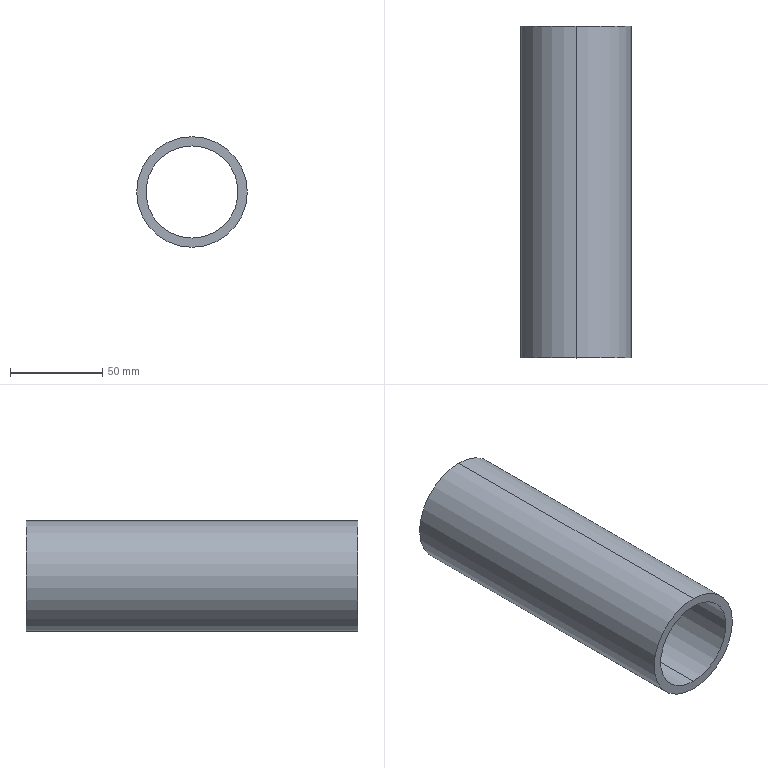Part | SolidWorks | features Extrusion 1 | 1 solid | 6 faces | box 60 x 180 x 60 mm | volume 155509 mm3 | cylinder 4 | plane 2 | commonest cylinder face diameters 50 x2 60 x2
STEP:
#1=CARTESIAN_POINT('',(0.,90.,-25.));
#2=VERTEX_POINT('',#1);
#3=CARTESIAN_POINT('',(0.,90.,25.));
#4=VERTEX_POINT('',#3);
#5=CARTESIAN_POINT('',(0.,90.,0.));
#6=DIRECTION('',(0.,1.,0.));
#7=DIRECTION('',(0.,0.,1.));
#8=AXIS2_PLACEMENT_3D('',#5,#6,#7);
#9=CIRCLE('',#8,25.);
#10=EDGE_CURVE('',#2,#4,#9,.T.);
#11=ORIENTED_EDGE('',*,*,#10,.T.);
#12=CARTESIAN_POINT('',(0.,-90.,25.));
#13=VERTEX_POINT('',#12);
#14=CARTESIAN_POINT('',(0.,90.,25.));
#15=DIRECTION('',(0.,-1.,0.));
#16=VECTOR('',#15,1000.);
#17=LINE('',#14,#16);
#18=EDGE_CURVE('',#4,#13,#17,.T.);
#19=ORIENTED_EDGE('',*,*,#18,.T.);
#20=CARTESIAN_POINT('',(0.,-90.,-25.));
#21=VERTEX_POINT('',#20);
#22=CARTESIAN_POINT('',(0.,-90.,0.));
#23=DIRECTION('',(0.,1.,0.));
#24=DIRECTION('',(0.,0.,1.));
#25=AXIS2_PLACEMENT_3D('',#22,#23,#24);
#26=CIRCLE('',#25,25.);
#27=EDGE_CURVE('',#21,#13,#26,.T.);
#28=ORIENTED_EDGE('',*,*,#27,.F.);
#29=CARTESIAN_POINT('',(0.,90.,-25.));
#30=DIRECTION('',(0.,-1.,0.));
#31=VECTOR('',#30,1000.);
#32=LINE('',#29,#31);
#33=EDGE_CURVE('',#2,#21,#32,.T.);
#34=ORIENTED_EDGE('',*,*,#33,.F.);
#35=EDGE_LOOP('',(#11,#19,#28,#34));
#36=FACE_OUTER_BOUND('',#35,.T.);
#37=CARTESIAN_POINT('',(0.,90.,0.));
#38=DIRECTION('',(0.,-1.,0.));
#39=DIRECTION('',(0.,0.,-1.));
#40=AXIS2_PLACEMENT_3D('',#37,#38,#39);
#41=CYLINDRICAL_SURFACE('',#40,25.);
#42=ADVANCED_FACE('',(#36),#41,.F.);
#43=CARTESIAN_POINT('',(0.,90.,30.));
#44=VERTEX_POINT('',#43);
#45=CARTESIAN_POINT('',(0.,90.,-30.));
#46=VERTEX_POINT('',#45);
#47=CARTESIAN_POINT('',(0.,90.,0.));
#48=DIRECTION('',(0.,1.,0.));
#49=DIRECTION('',(0.,0.,1.));
#50=AXIS2_PLACEMENT_3D('',#47,#48,#49);
#51=CIRCLE('',#50,30.);
#52=EDGE_CURVE('',#44,#46,#51,.T.);
#53=ORIENTED_EDGE('',*,*,#52,.F.);
#54=CARTESIAN_POINT('',(0.,-90.,30.));
#55=VERTEX_POINT('',#54);
#56=CARTESIAN_POINT('',(0.,90.,30.));
#57=DIRECTION('',(0.,-1.,0.));
#58=VECTOR('',#57,1000.);
#59=LINE('',#56,#58);
#60=EDGE_CURVE('',#44,#55,#59,.T.);
#61=ORIENTED_EDGE('',*,*,#60,.T.);
#62=CARTESIAN_POINT('',(0.,-90.,-30.));
#63=VERTEX_POINT('',#62);
#64=CARTESIAN_POINT('',(0.,-90.,0.));
#65=DIRECTION('',(0.,1.,0.));
#66=DIRECTION('',(0.,0.,1.));
#67=AXIS2_PLACEMENT_3D('',#64,#65,#66);
#68=CIRCLE('',#67,30.);
#69=EDGE_CURVE('',#55,#63,#68,.T.);
#70=ORIENTED_EDGE('',*,*,#69,.T.);
#71=CARTESIAN_POINT('',(0.,90.,-30.));
#72=DIRECTION('',(0.,-1.,0.));
#73=VECTOR('',#72,1000.);
#74=LINE('',#71,#73);
#75=EDGE_CURVE('',#46,#63,#74,.T.);
#76=ORIENTED_EDGE('',*,*,#75,.F.);
#77=EDGE_LOOP('',(#53,#61,#70,#76));
#78=FACE_OUTER_BOUND('',#77,.T.);
#79=CARTESIAN_POINT('',(0.,90.,0.));
#80=DIRECTION('',(0.,-1.,0.));
#81=DIRECTION('',(0.,0.,-1.));
#82=AXIS2_PLACEMENT_3D('',#79,#80,#81);
#83=CYLINDRICAL_SURFACE('',#82,30.);
#84=ADVANCED_FACE('',(#78),#83,.T.);
#85=CARTESIAN_POINT('',(0.,90.,0.));
#86=DIRECTION('',(0.,1.,0.));
#87=DIRECTION('',(0.,0.,1.));
#88=AXIS2_PLACEMENT_3D('',#85,#86,#87);
#89=CIRCLE('',#88,30.);
#90=EDGE_CURVE('',#46,#44,#89,.T.);
#91=ORIENTED_EDGE('',*,*,#90,.T.);
#92=ORIENTED_EDGE('',*,*,#52,.T.);
#93=EDGE_LOOP('',(#91,#92));
#94=FACE_OUTER_BOUND('',#93,.T.);
#95=ORIENTED_EDGE('',*,*,#10,.F.);
#96=CARTESIAN_POINT('',(0.,90.,0.));
#97=DIRECTION('',(0.,1.,0.));
#98=DIRECTION('',(0.,0.,1.));
#99=AXIS2_PLACEMENT_3D('',#96,#97,#98);
#100=CIRCLE('',#99,25.);
#101=EDGE_CURVE('',#4,#2,#100,.T.);
#102=ORIENTED_EDGE('',*,*,#101,.F.);
#103=EDGE_LOOP('',(#95,#102));
#104=FACE_BOUND('',#103,.T.);
#105=CARTESIAN_POINT('',(0.,90.,0.));
#106=DIRECTION('',(0.,1.,0.));
#107=DIRECTION('',(0.,0.,1.));
#108=AXIS2_PLACEMENT_3D('',#105,#106,#107);
#109=PLANE('',#108);
#110=ADVANCED_FACE('',(#94,#104),#109,.T.);
#111=CARTESIAN_POINT('',(0.,-90.,0.));
#112=DIRECTION('',(0.,1.,0.));
#113=DIRECTION('',(0.,0.,1.));
#114=AXIS2_PLACEMENT_3D('',#111,#112,#113);
#115=CIRCLE('',#114,30.);
#116=EDGE_CURVE('',#63,#55,#115,.T.);
#117=ORIENTED_EDGE('',*,*,#116,.F.);
#118=ORIENTED_EDGE('',*,*,#69,.F.);
#119=EDGE_LOOP('',(#117,#118));
#120=FACE_OUTER_BOUND('',#119,.T.);
#121=ORIENTED_EDGE('',*,*,#27,.T.);
#122=CARTESIAN_POINT('',(0.,-90.,0.));
#123=DIRECTION('',(0.,1.,0.));
#124=DIRECTION('',(0.,0.,1.));
#125=AXIS2_PLACEMENT_3D('',#122,#123,#124);
#126=CIRCLE('',#125,25.);
#127=EDGE_CURVE('',#13,#21,#126,.T.);
#128=ORIENTED_EDGE('',*,*,#127,.T.);
#129=EDGE_LOOP('',(#121,#128));
#130=FACE_BOUND('',#129,.T.);
#131=CARTESIAN_POINT('',(0.,-90.,0.));
#132=DIRECTION('',(0.,1.,0.));
#133=DIRECTION('',(0.,0.,1.));
#134=AXIS2_PLACEMENT_3D('',#131,#132,#133);
#135=PLANE('',#134);
#136=ADVANCED_FACE('',(#120,#130),#135,.F.);
#137=ORIENTED_EDGE('',*,*,#60,.F.);
#138=ORIENTED_EDGE('',*,*,#90,.F.);
#139=ORIENTED_EDGE('',*,*,#75,.T.);
#140=ORIENTED_EDGE('',*,*,#116,.T.);
#141=EDGE_LOOP('',(#137,#138,#139,#140));
#142=FACE_OUTER_BOUND('',#141,.T.);
#143=CARTESIAN_POINT('',(0.,90.,0.));
#144=DIRECTION('',(0.,-1.,0.));
#145=DIRECTION('',(0.,0.,-1.));
#146=AXIS2_PLACEMENT_3D('',#143,#144,#145);
#147=CYLINDRICAL_SURFACE('',#146,30.);
#148=ADVANCED_FACE('',(#142),#147,.T.);
#149=ORIENTED_EDGE('',*,*,#18,.F.);
#150=ORIENTED_EDGE('',*,*,#101,.T.);
#151=ORIENTED_EDGE('',*,*,#33,.T.);
#152=ORIENTED_EDGE('',*,*,#127,.F.);
#153=EDGE_LOOP('',(#149,#150,#151,#152));
#154=FACE_OUTER_BOUND('',#153,.T.);
#155=CARTESIAN_POINT('',(0.,90.,0.));
#156=DIRECTION('',(0.,-1.,0.));
#157=DIRECTION('',(0.,0.,-1.));
#158=AXIS2_PLACEMENT_3D('',#155,#156,#157);
#159=CYLINDRICAL_SURFACE('',#158,25.);
#160=ADVANCED_FACE('',(#154),#159,.F.);
#161=CLOSED_SHELL('',(#42,#84,#110,#136,#148,#160));
#162=MANIFOLD_SOLID_BREP('',#161);
#163=CARTESIAN_POINT('',(0.,0.,0.));
#164=DIRECTION('',(0.,0.,1.));
#165=DIRECTION('',(1.,0.,0.));
#166=AXIS2_PLACEMENT_3D('',#163,#164,#165);
#167=(LENGTH_UNIT()NAMED_UNIT(*)SI_UNIT(.MILLI.,.METRE.));
#168=UNCERTAINTY_MEASURE_WITH_UNIT(LENGTH_MEASURE(0.00001),#167,'','');
#169=(NAMED_UNIT(*)PLANE_ANGLE_UNIT()SI_UNIT($,.RADIAN.));
#170=(NAMED_UNIT(*)SI_UNIT($,.STERADIAN.)SOLID_ANGLE_UNIT());
#171=(GEOMETRIC_REPRESENTATION_CONTEXT(3)GLOBAL_UNCERTAINTY_ASSIGNED_CONTEXT((#168))GLOBAL_UNIT_ASSIGNED_CONTEXT((#167,#169,#170))REPRESENTATION_CONTEXT('',''));
#172=ADVANCED_BREP_SHAPE_REPRESENTATION('',(#162,#166),#171);